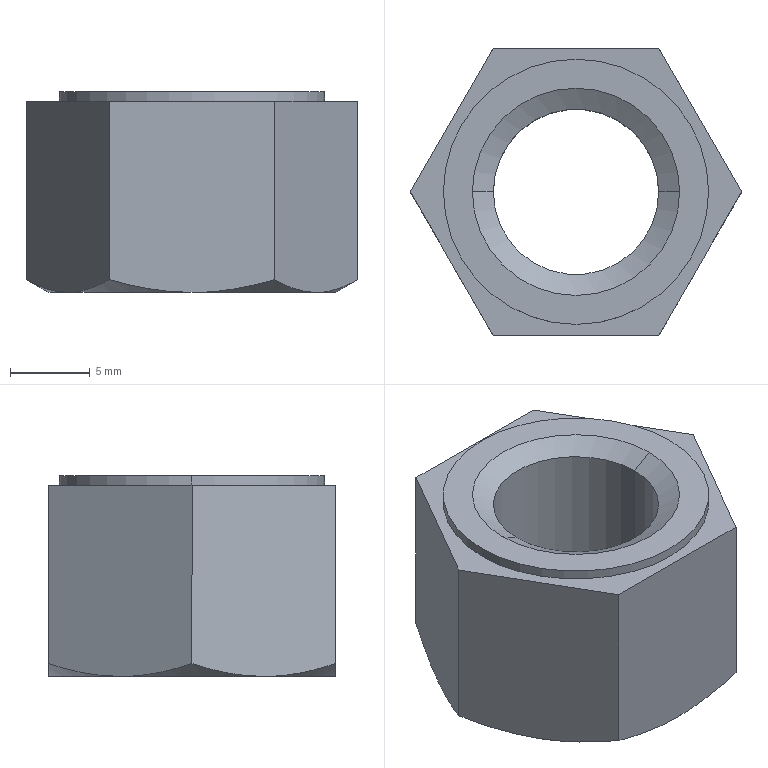Part | SolidWorks | features RevCut 4, Chamfer 2, Boss 1, Extrusion 1, LPattern 1 | 1 solid | 24 faces | box 20.785 x 18 x 12.6 mm | volume 2391 mm3 | cone 11 | plane 9 | cylinder 4 | commonest cylinder face diameters 10.376 x2 16.63 x2
STEP:
#1=CARTESIAN_POINT('',(-5.188,0.,-0.1575));
#2=VERTEX_POINT('',#1);
#3=CARTESIAN_POINT('',(5.188,0.,-0.1575));
#4=VERTEX_POINT('',#3);
#5=CARTESIAN_POINT('',(0.,0.,-0.1575));
#6=DIRECTION('',(0.,0.,1.));
#7=DIRECTION('',(1.,0.,0.));
#8=AXIS2_PLACEMENT_3D('',#5,#6,#7);
#9=CIRCLE('',#8,5.188);
#10=EDGE_CURVE('',#2,#4,#9,.T.);
#11=ORIENTED_EDGE('',*,*,#10,.F.);
#12=CARTESIAN_POINT('',(-6.5,0.,0.6));
#13=VERTEX_POINT('',#12);
#14=CARTESIAN_POINT('',(-5.188,0.,-0.1575));
#15=DIRECTION('',(-0.866,0.,0.5));
#16=VECTOR('',#15,1000.);
#17=LINE('',#14,#16);
#18=EDGE_CURVE('',#2,#13,#17,.T.);
#19=ORIENTED_EDGE('',*,*,#18,.T.);
#20=CARTESIAN_POINT('',(6.5,0.,0.6));
#21=VERTEX_POINT('',#20);
#22=CARTESIAN_POINT('',(0.,0.,0.6));
#23=DIRECTION('',(0.,0.,-1.));
#24=DIRECTION('',(1.,0.,0.));
#25=AXIS2_PLACEMENT_3D('',#22,#23,#24);
#26=CIRCLE('',#25,6.5);
#27=EDGE_CURVE('',#21,#13,#26,.T.);
#28=ORIENTED_EDGE('',*,*,#27,.F.);
#29=CARTESIAN_POINT('',(5.188,0.,-0.1575));
#30=DIRECTION('',(0.866,0.,0.5));
#31=VECTOR('',#30,1000.);
#32=LINE('',#29,#31);
#33=EDGE_CURVE('',#4,#21,#32,.T.);
#34=ORIENTED_EDGE('',*,*,#33,.F.);
#35=EDGE_LOOP('',(#11,#19,#28,#34));
#36=FACE_OUTER_BOUND('',#35,.T.);
#37=CARTESIAN_POINT('',(0.,0.,-0.1575));
#38=DIRECTION('',(0.,0.,1.));
#39=DIRECTION('',(1.,0.,0.));
#40=AXIS2_PLACEMENT_3D('',#37,#38,#39);
#41=CONICAL_SURFACE('',#40,5.188,1.047);
#42=ADVANCED_FACE('',(#36),#41,.F.);
#43=CARTESIAN_POINT('',(8.315,0.,0.6));
#44=VERTEX_POINT('',#43);
#45=CARTESIAN_POINT('',(-8.315,0.,0.6));
#46=VERTEX_POINT('',#45);
#47=CARTESIAN_POINT('',(0.,0.,0.6));
#48=DIRECTION('',(0.,0.,1.));
#49=DIRECTION('',(1.,0.,0.));
#50=AXIS2_PLACEMENT_3D('',#47,#48,#49);
#51=CIRCLE('',#50,8.315);
#52=EDGE_CURVE('',#44,#46,#51,.T.);
#53=ORIENTED_EDGE('',*,*,#52,.F.);
#54=CARTESIAN_POINT('',(8.315,0.,0.));
#55=VERTEX_POINT('',#54);
#56=CARTESIAN_POINT('',(8.315,0.,0.6));
#57=DIRECTION('',(0.,0.,-1.));
#58=VECTOR('',#57,1000.);
#59=LINE('',#56,#58);
#60=EDGE_CURVE('',#44,#55,#59,.T.);
#61=ORIENTED_EDGE('',*,*,#60,.T.);
#62=CARTESIAN_POINT('',(-8.315,0.,0.));
#63=VERTEX_POINT('',#62);
#64=CARTESIAN_POINT('',(0.,0.,0.));
#65=DIRECTION('',(0.,0.,1.));
#66=DIRECTION('',(1.,0.,0.));
#67=AXIS2_PLACEMENT_3D('',#64,#65,#66);
#68=CIRCLE('',#67,8.315);
#69=EDGE_CURVE('',#55,#63,#68,.T.);
#70=ORIENTED_EDGE('',*,*,#69,.T.);
#71=CARTESIAN_POINT('',(-8.315,0.,0.6));
#72=DIRECTION('',(0.,0.,-1.));
#73=VECTOR('',#72,1000.);
#74=LINE('',#71,#73);
#75=EDGE_CURVE('',#46,#63,#74,.T.);
#76=ORIENTED_EDGE('',*,*,#75,.F.);
#77=EDGE_LOOP('',(#53,#61,#70,#76));
#78=FACE_OUTER_BOUND('',#77,.T.);
#79=CARTESIAN_POINT('',(0.,0.,0.6));
#80=DIRECTION('',(0.,0.,-1.));
#81=DIRECTION('',(-1.,0.,0.));
#82=AXIS2_PLACEMENT_3D('',#79,#80,#81);
#83=CYLINDRICAL_SURFACE('',#82,8.315);
#84=ADVANCED_FACE('',(#78),#83,.T.);
#85=CARTESIAN_POINT('',(-5.188,0.,-11.243));
#86=VERTEX_POINT('',#85);
#87=CARTESIAN_POINT('',(5.188,0.,-11.243));
#88=VERTEX_POINT('',#87);
#89=CARTESIAN_POINT('',(0.,0.,-11.243));
#90=DIRECTION('',(0.,0.,1.));
#91=DIRECTION('',(1.,0.,0.));
#92=AXIS2_PLACEMENT_3D('',#89,#90,#91);
#93=CIRCLE('',#92,5.188);
#94=EDGE_CURVE('',#86,#88,#93,.T.);
#95=ORIENTED_EDGE('',*,*,#94,.T.);
#96=CARTESIAN_POINT('',(6.5,0.,-12.));
#97=VERTEX_POINT('',#96);
#98=CARTESIAN_POINT('',(5.188,0.,-11.243));
#99=DIRECTION('',(0.866,0.,-0.5));
#100=VECTOR('',#99,1000.);
#101=LINE('',#98,#100);
#102=EDGE_CURVE('',#88,#97,#101,.T.);
#103=ORIENTED_EDGE('',*,*,#102,.T.);
#104=CARTESIAN_POINT('',(-6.5,0.,-12.));
#105=VERTEX_POINT('',#104);
#106=CARTESIAN_POINT('',(0.,0.,-12.));
#107=DIRECTION('',(0.,0.,1.));
#108=DIRECTION('',(1.,0.,0.));
#109=AXIS2_PLACEMENT_3D('',#106,#107,#108);
#110=CIRCLE('',#109,6.5);
#111=EDGE_CURVE('',#105,#97,#110,.T.);
#112=ORIENTED_EDGE('',*,*,#111,.F.);
#113=CARTESIAN_POINT('',(-5.188,0.,-11.243));
#114=DIRECTION('',(-0.866,0.,-0.5));
#115=VECTOR('',#114,1000.);
#116=LINE('',#113,#115);
#117=EDGE_CURVE('',#86,#105,#116,.T.);
#118=ORIENTED_EDGE('',*,*,#117,.F.);
#119=EDGE_LOOP('',(#95,#103,#112,#118));
#120=FACE_OUTER_BOUND('',#119,.T.);
#121=CARTESIAN_POINT('',(0.,0.,-11.243));
#122=DIRECTION('',(0.,0.,-1.));
#123=DIRECTION('',(-1.,0.,0.));
#124=AXIS2_PLACEMENT_3D('',#121,#122,#123);
#125=CONICAL_SURFACE('',#124,5.188,1.047);
#126=ADVANCED_FACE('',(#120),#125,.F.);
#127=CARTESIAN_POINT('',(7.794,-4.5,-12.));
#128=VERTEX_POINT('',#127);
#129=CARTESIAN_POINT('',(9.,0.,-12.));
#130=VERTEX_POINT('',#129);
#131=CARTESIAN_POINT('',(0.,0.,-12.));
#132=DIRECTION('',(0.,0.,1.));
#133=DIRECTION('',(1.,0.,0.));
#134=AXIS2_PLACEMENT_3D('',#131,#132,#133);
#135=CIRCLE('',#134,9.);
#136=EDGE_CURVE('',#128,#130,#135,.T.);
#137=ORIENTED_EDGE('',*,*,#136,.T.);
#138=CARTESIAN_POINT('',(10.392,0.,-11.196));
#139=VERTEX_POINT('',#138);
#140=CARTESIAN_POINT('',(9.,0.,-12.));
#141=DIRECTION('',(0.866,0.,0.5));
#142=VECTOR('',#141,1000.);
#143=LINE('',#140,#142);
#144=EDGE_CURVE('',#130,#139,#143,.T.);
#145=ORIENTED_EDGE('',*,*,#144,.T.);
#146=CARTESIAN_POINT('',(7.794,-4.5,-12.));
#147=CARTESIAN_POINT('',(8.015,-4.118,-12.));
#148=CARTESIAN_POINT('',(8.236,-3.734,-11.981));
#149=CARTESIAN_POINT('',(8.674,-2.976,-11.907));
#150=CARTESIAN_POINT('',(8.892,-2.599,-11.853));
#151=CARTESIAN_POINT('',(9.541,-1.475,-11.643));
#152=CARTESIAN_POINT('',(9.968,-0.7343,-11.441));
#153=CARTESIAN_POINT('',(10.392,0.,-11.196));
#154=B_SPLINE_CURVE_WITH_KNOTS('',3,(#146,#147,#148,#149,#150,#151,#152,#153),.UNSPECIFIED.,.F.,.F.,(4,2,2,4),(0.005258,0.006567,0.007877,0.0105),.UNSPECIFIED.);
#155=EDGE_CURVE('',#128,#139,#154,.T.);
#156=ORIENTED_EDGE('',*,*,#155,.F.);
#157=EDGE_LOOP('',(#137,#145,#156));
#158=FACE_OUTER_BOUND('',#157,.T.);
#159=CARTESIAN_POINT('',(0.,0.,-12.));
#160=DIRECTION('',(0.,0.,1.));
#161=DIRECTION('',(1.,0.,0.));
#162=AXIS2_PLACEMENT_3D('',#159,#160,#161);
#163=CONICAL_SURFACE('',#162,9.,1.047);
#164=ADVANCED_FACE('',(#158),#163,.T.);
#165=ORIENTED_EDGE('',*,*,#94,.F.);
#166=CARTESIAN_POINT('',(-5.188,0.,-12.));
#167=DIRECTION('',(0.,0.,1.));
#168=VECTOR('',#167,1000.);
#169=LINE('',#166,#168);
#170=EDGE_CURVE('',#86,#2,#169,.T.);
#171=ORIENTED_EDGE('',*,*,#170,.T.);
#172=ORIENTED_EDGE('',*,*,#10,.T.);
#173=CARTESIAN_POINT('',(5.188,0.,-12.));
#174=DIRECTION('',(0.,0.,1.));
#175=VECTOR('',#174,1000.);
#176=LINE('',#173,#175);
#177=EDGE_CURVE('',#88,#4,#176,.T.);
#178=ORIENTED_EDGE('',*,*,#177,.F.);
#179=EDGE_LOOP('',(#165,#171,#172,#178));
#180=FACE_OUTER_BOUND('',#179,.T.);
#181=CARTESIAN_POINT('',(0.,0.,-12.));
#182=DIRECTION('',(0.,0.,1.));
#183=DIRECTION('',(1.,0.,0.));
#184=AXIS2_PLACEMENT_3D('',#181,#182,#183);
#185=CYLINDRICAL_SURFACE('',#184,5.188);
#186=ADVANCED_FACE('',(#180),#185,.F.);
#187=CARTESIAN_POINT('',(-5.196,-9.,0.));
#188=VERTEX_POINT('',#187);
#189=CARTESIAN_POINT('',(5.196,-9.,0.));
#190=VERTEX_POINT('',#189);
#191=CARTESIAN_POINT('',(-5.196,-9.,0.));
#192=DIRECTION('',(1.,0.,0.));
#193=VECTOR('',#192,1000.);
#194=LINE('',#191,#193);
#195=EDGE_CURVE('',#188,#190,#194,.T.);
#196=ORIENTED_EDGE('',*,*,#195,.T.);
#197=CARTESIAN_POINT('',(10.392,0.,0.));
#198=VERTEX_POINT('',#197);
#199=CARTESIAN_POINT('',(5.196,-9.,0.));
#200=DIRECTION('',(0.5,0.866,0.));
#201=VECTOR('',#200,1000.);
#202=LINE('',#199,#201);
#203=EDGE_CURVE('',#190,#198,#202,.T.);
#204=ORIENTED_EDGE('',*,*,#203,.T.);
#205=CARTESIAN_POINT('',(5.196,9.,0.));
#206=VERTEX_POINT('',#205);
#207=CARTESIAN_POINT('',(10.392,0.,0.));
#208=DIRECTION('',(-0.5,0.866,0.));
#209=VECTOR('',#208,1000.);
#210=LINE('',#207,#209);
#211=EDGE_CURVE('',#198,#206,#210,.T.);
#212=ORIENTED_EDGE('',*,*,#211,.T.);
#213=CARTESIAN_POINT('',(-5.196,9.,0.));
#214=VERTEX_POINT('',#213);
#215=CARTESIAN_POINT('',(5.196,9.,0.));
#216=DIRECTION('',(-1.,0.,0.));
#217=VECTOR('',#216,1000.);
#218=LINE('',#215,#217);
#219=EDGE_CURVE('',#206,#214,#218,.T.);
#220=ORIENTED_EDGE('',*,*,#219,.T.);
#221=CARTESIAN_POINT('',(-10.392,0.,0.));
#222=VERTEX_POINT('',#221);
#223=CARTESIAN_POINT('',(-5.196,9.,0.));
#224=DIRECTION('',(-0.5,-0.866,0.));
#225=VECTOR('',#224,1000.);
#226=LINE('',#223,#225);
#227=EDGE_CURVE('',#214,#222,#226,.T.);
#228=ORIENTED_EDGE('',*,*,#227,.T.);
#229=CARTESIAN_POINT('',(-10.392,0.,0.));
#230=DIRECTION('',(0.5,-0.866,0.));
#231=VECTOR('',#230,1000.);
#232=LINE('',#229,#231);
#233=EDGE_CURVE('',#222,#188,#232,.T.);
#234=ORIENTED_EDGE('',*,*,#233,.T.);
#235=EDGE_LOOP('',(#196,#204,#212,#220,#228,#234));
#236=FACE_OUTER_BOUND('',#235,.T.);
#237=CARTESIAN_POINT('',(0.,0.,0.));
#238=DIRECTION('',(0.,0.,1.));
#239=DIRECTION('',(1.,0.,0.));
#240=AXIS2_PLACEMENT_3D('',#237,#238,#239);
#241=CIRCLE('',#240,8.315);
#242=EDGE_CURVE('',#63,#55,#241,.T.);
#243=ORIENTED_EDGE('',*,*,#242,.F.);
#244=ORIENTED_EDGE('',*,*,#69,.F.);
#245=EDGE_LOOP('',(#243,#244));
#246=FACE_BOUND('',#245,.T.);
#247=CARTESIAN_POINT('',(5.196,-9.,0.));
#248=DIRECTION('',(0.,0.,1.));
#249=DIRECTION('',(1.,0.,0.));
#250=AXIS2_PLACEMENT_3D('',#247,#248,#249);
#251=PLANE('',#250);
#252=ADVANCED_FACE('',(#236,#246),#251,.T.);
#253=CARTESIAN_POINT('',(-5.196,-9.,-11.196));
#254=VERTEX_POINT('',#253);
#255=CARTESIAN_POINT('',(-5.196,-9.,-12.));
#256=DIRECTION('',(0.,0.,1.));
#257=VECTOR('',#256,1000.);
#258=LINE('',#255,#257);
#259=EDGE_CURVE('',#254,#188,#258,.T.);
#260=ORIENTED_EDGE('',*,*,#259,.F.);
#261=CARTESIAN_POINT('',(0.,-9.,-12.));
#262=VERTEX_POINT('',#261);
#263=CARTESIAN_POINT('',(-5.196,-9.,-11.196));
#264=CARTESIAN_POINT('',(-4.351,-9.,-11.44));
#265=CARTESIAN_POINT('',(-3.485,-9.,-11.645));
#266=CARTESIAN_POINT('',(-1.75,-9.,-11.925));
#267=CARTESIAN_POINT('',(-0.8781,-9.,-12.));
#268=CARTESIAN_POINT('',(0.,-9.,-12.));
#269=B_SPLINE_CURVE_WITH_KNOTS('',3,(#263,#264,#265,#266,#267,#268),.UNSPECIFIED.,.F.,.F.,(4,2,4),(0.009271,0.0119,0.01453),.UNSPECIFIED.);
#270=EDGE_CURVE('',#254,#262,#269,.T.);
#271=ORIENTED_EDGE('',*,*,#270,.T.);
#272=CARTESIAN_POINT('',(5.196,-9.,-11.196));
#273=VERTEX_POINT('',#272);
#274=CARTESIAN_POINT('',(0.,-9.,-12.));
#275=CARTESIAN_POINT('',(0.8786,-9.,-12.));
#276=CARTESIAN_POINT('',(1.769,-9.,-11.922));
#277=CARTESIAN_POINT('',(3.505,-9.,-11.641));
#278=CARTESIAN_POINT('',(4.356,-9.,-11.439));
#279=CARTESIAN_POINT('',(5.196,-9.,-11.196));
#280=B_SPLINE_CURVE_WITH_KNOTS('',3,(#274,#275,#276,#277,#278,#279),.UNSPECIFIED.,.F.,.F.,(4,2,4),(0.01453,0.01716,0.01979),.UNSPECIFIED.);
#281=EDGE_CURVE('',#262,#273,#280,.T.);
#282=ORIENTED_EDGE('',*,*,#281,.T.);
#283=CARTESIAN_POINT('',(5.196,-9.,-12.));
#284=DIRECTION('',(0.,0.,1.));
#285=VECTOR('',#284,1000.);
#286=LINE('',#283,#285);
#287=EDGE_CURVE('',#273,#190,#286,.T.);
#288=ORIENTED_EDGE('',*,*,#287,.T.);
#289=ORIENTED_EDGE('',*,*,#195,.F.);
#290=EDGE_LOOP('',(#260,#271,#282,#288,#289));
#291=FACE_OUTER_BOUND('',#290,.T.);
#292=CARTESIAN_POINT('',(-5.196,-9.,-12.));
#293=DIRECTION('',(0.,-1.,0.));
#294=DIRECTION('',(1.,0.,0.));
#295=AXIS2_PLACEMENT_3D('',#292,#293,#294);
#296=PLANE('',#295);
#297=ADVANCED_FACE('',(#291),#296,.T.);
#298=CARTESIAN_POINT('',(-10.392,0.,-11.196));
#299=VERTEX_POINT('',#298);
#300=CARTESIAN_POINT('',(-10.392,0.,-12.));
#301=DIRECTION('',(0.,0.,1.));
#302=VECTOR('',#301,1000.);
#303=LINE('',#300,#302);
#304=EDGE_CURVE('',#299,#222,#303,.T.);
#305=ORIENTED_EDGE('',*,*,#304,.F.);
#306=CARTESIAN_POINT('',(-7.794,-4.5,-12.));
#307=VERTEX_POINT('',#306);
#308=CARTESIAN_POINT('',(-10.392,0.,-11.196));
#309=CARTESIAN_POINT('',(-9.967,-0.7361,-11.442));
#310=CARTESIAN_POINT('',(-9.539,-1.478,-11.644));
#311=CARTESIAN_POINT('',(-8.674,-2.976,-11.923));
#312=CARTESIAN_POINT('',(-8.237,-3.733,-12.));
#313=CARTESIAN_POINT('',(-7.794,-4.5,-12.));
#314=B_SPLINE_CURVE_WITH_KNOTS('',3,(#308,#309,#310,#311,#312,#313),.UNSPECIFIED.,.F.,.F.,(4,2,4),(0.000000238,0.002629,0.005258),.UNSPECIFIED.);
#315=EDGE_CURVE('',#299,#307,#314,.T.);
#316=ORIENTED_EDGE('',*,*,#315,.T.);
#317=CARTESIAN_POINT('',(-7.794,-4.5,-12.));
#318=CARTESIAN_POINT('',(-7.574,-4.882,-12.));
#319=CARTESIAN_POINT('',(-7.352,-5.266,-11.981));
#320=CARTESIAN_POINT('',(-6.914,-6.024,-11.907));
#321=CARTESIAN_POINT('',(-6.697,-6.401,-11.853));
#322=CARTESIAN_POINT('',(-6.048,-7.525,-11.643));
#323=CARTESIAN_POINT('',(-5.62,-8.266,-11.441));
#324=CARTESIAN_POINT('',(-5.196,-9.,-11.196));
#325=B_SPLINE_CURVE_WITH_KNOTS('',3,(#317,#318,#319,#320,#321,#322,#323,#324),.UNSPECIFIED.,.F.,.F.,(4,2,2,4),(0.005258,0.006567,0.007877,0.0105),.UNSPECIFIED.);
#326=EDGE_CURVE('',#307,#254,#325,.T.);
#327=ORIENTED_EDGE('',*,*,#326,.T.);
#328=ORIENTED_EDGE('',*,*,#259,.T.);
#329=ORIENTED_EDGE('',*,*,#233,.F.);
#330=EDGE_LOOP('',(#305,#316,#327,#328,#329));
#331=FACE_OUTER_BOUND('',#330,.T.);
#332=CARTESIAN_POINT('',(-10.392,0.,-12.));
#333=DIRECTION('',(-0.866,-0.5,0.));
#334=DIRECTION('',(0.5,-0.866,0.));
#335=AXIS2_PLACEMENT_3D('',#332,#333,#334);
#336=PLANE('',#335);
#337=ADVANCED_FACE('',(#331),#336,.T.);
#338=CARTESIAN_POINT('',(-5.196,9.,-11.196));
#339=VERTEX_POINT('',#338);
#340=CARTESIAN_POINT('',(-5.196,9.,-12.));
#341=DIRECTION('',(0.,0.,1.));
#342=VECTOR('',#341,1000.);
#343=LINE('',#340,#342);
#344=EDGE_CURVE('',#339,#214,#343,.T.);
#345=ORIENTED_EDGE('',*,*,#344,.F.);
#346=CARTESIAN_POINT('',(-7.794,4.5,-12.));
#347=VERTEX_POINT('',#346);
#348=CARTESIAN_POINT('',(-5.196,9.,-11.196));
#349=CARTESIAN_POINT('',(-5.621,8.264,-11.442));
#350=CARTESIAN_POINT('',(-6.049,7.522,-11.644));
#351=CARTESIAN_POINT('',(-6.914,6.024,-11.923));
#352=CARTESIAN_POINT('',(-7.352,5.267,-12.));
#353=CARTESIAN_POINT('',(-7.794,4.5,-12.));
#354=B_SPLINE_CURVE_WITH_KNOTS('',3,(#348,#349,#350,#351,#352,#353),.UNSPECIFIED.,.F.,.F.,(4,2,4),(0.000000238,0.002629,0.005258),.UNSPECIFIED.);
#355=EDGE_CURVE('',#339,#347,#354,.T.);
#356=ORIENTED_EDGE('',*,*,#355,.T.);
#357=CARTESIAN_POINT('',(-7.794,4.5,-12.));
#358=CARTESIAN_POINT('',(-8.015,4.118,-12.));
#359=CARTESIAN_POINT('',(-8.236,3.734,-11.981));
#360=CARTESIAN_POINT('',(-8.674,2.976,-11.907));
#361=CARTESIAN_POINT('',(-8.892,2.599,-11.853));
#362=CARTESIAN_POINT('',(-9.541,1.475,-11.643));
#363=CARTESIAN_POINT('',(-9.968,0.7343,-11.441));
#364=CARTESIAN_POINT('',(-10.392,0.,-11.196));
#365=B_SPLINE_CURVE_WITH_KNOTS('',3,(#357,#358,#359,#360,#361,#362,#363,#364),.UNSPECIFIED.,.F.,.F.,(4,2,2,4),(0.005258,0.006567,0.007877,0.0105),.UNSPECIFIED.);
#366=EDGE_CURVE('',#347,#299,#365,.T.);
#367=ORIENTED_EDGE('',*,*,#366,.T.);
#368=ORIENTED_EDGE('',*,*,#304,.T.);
#369=ORIENTED_EDGE('',*,*,#227,.F.);
#370=EDGE_LOOP('',(#345,#356,#367,#368,#369));
#371=FACE_OUTER_BOUND('',#370,.T.);
#372=CARTESIAN_POINT('',(-5.196,9.,-12.));
#373=DIRECTION('',(-0.866,0.5,0.));
#374=DIRECTION('',(-0.5,-0.866,0.));
#375=AXIS2_PLACEMENT_3D('',#372,#373,#374);
#376=PLANE('',#375);
#377=ADVANCED_FACE('',(#371),#376,.T.);
#378=CARTESIAN_POINT('',(5.196,9.,-11.196));
#379=VERTEX_POINT('',#378);
#380=CARTESIAN_POINT('',(5.196,9.,-12.));
#381=DIRECTION('',(0.,0.,1.));
#382=VECTOR('',#381,1000.);
#383=LINE('',#380,#382);
#384=EDGE_CURVE('',#379,#206,#383,.T.);
#385=ORIENTED_EDGE('',*,*,#384,.F.);
#386=CARTESIAN_POINT('',(0.,9.,-12.));
#387=VERTEX_POINT('',#386);
#388=CARTESIAN_POINT('',(5.196,9.,-11.196));
#389=CARTESIAN_POINT('',(4.356,9.,-11.439));
#390=CARTESIAN_POINT('',(3.505,9.,-11.641));
#391=CARTESIAN_POINT('',(1.769,9.,-11.922));
#392=CARTESIAN_POINT('',(0.8786,9.,-12.));
#393=CARTESIAN_POINT('',(0.,9.,-12.));
#394=B_SPLINE_CURVE_WITH_KNOTS('',3,(#388,#389,#390,#391,#392,#393),.UNSPECIFIED.,.F.,.F.,(4,2,4),(0.003809,0.006432,0.009055),.UNSPECIFIED.);
#395=EDGE_CURVE('',#379,#387,#394,.T.);
#396=ORIENTED_EDGE('',*,*,#395,.T.);
#397=CARTESIAN_POINT('',(0.,9.,-12.));
#398=CARTESIAN_POINT('',(-0.8781,9.,-12.));
#399=CARTESIAN_POINT('',(-1.75,9.,-11.925));
#400=CARTESIAN_POINT('',(-3.485,9.,-11.645));
#401=CARTESIAN_POINT('',(-4.351,9.,-11.44));
#402=CARTESIAN_POINT('',(-5.196,9.,-11.196));
#403=B_SPLINE_CURVE_WITH_KNOTS('',3,(#397,#398,#399,#400,#401,#402),.UNSPECIFIED.,.F.,.F.,(4,2,4),(0.009055,0.01168,0.0143),.UNSPECIFIED.);
#404=EDGE_CURVE('',#387,#339,#403,.T.);
#405=ORIENTED_EDGE('',*,*,#404,.T.);
#406=ORIENTED_EDGE('',*,*,#344,.T.);
#407=ORIENTED_EDGE('',*,*,#219,.F.);
#408=EDGE_LOOP('',(#385,#396,#405,#406,#407));
#409=FACE_OUTER_BOUND('',#408,.T.);
#410=CARTESIAN_POINT('',(5.196,9.,-12.));
#411=DIRECTION('',(0.,1.,0.));
#412=DIRECTION('',(0.,0.,1.));
#413=AXIS2_PLACEMENT_3D('',#410,#411,#412);
#414=PLANE('',#413);
#415=ADVANCED_FACE('',(#409),#414,.T.);
#416=CARTESIAN_POINT('',(10.392,0.,-12.));
#417=DIRECTION('',(0.,0.,1.));
#418=VECTOR('',#417,1000.);
#419=LINE('',#416,#418);
#420=EDGE_CURVE('',#139,#198,#419,.T.);
#421=ORIENTED_EDGE('',*,*,#420,.F.);
#422=CARTESIAN_POINT('',(7.794,4.5,-12.));
#423=VERTEX_POINT('',#422);
#424=CARTESIAN_POINT('',(10.392,0.,-11.196));
#425=CARTESIAN_POINT('',(9.967,0.7361,-11.442));
#426=CARTESIAN_POINT('',(9.539,1.478,-11.644));
#427=CARTESIAN_POINT('',(8.674,2.976,-11.923));
#428=CARTESIAN_POINT('',(8.237,3.733,-12.));
#429=CARTESIAN_POINT('',(7.794,4.5,-12.));
#430=B_SPLINE_CURVE_WITH_KNOTS('',3,(#424,#425,#426,#427,#428,#429),.UNSPECIFIED.,.F.,.F.,(4,2,4),(0.000000238,0.002629,0.005258),.UNSPECIFIED.);
#431=EDGE_CURVE('',#139,#423,#430,.T.);
#432=ORIENTED_EDGE('',*,*,#431,.T.);
#433=CARTESIAN_POINT('',(7.794,4.5,-12.));
#434=CARTESIAN_POINT('',(7.574,4.882,-12.));
#435=CARTESIAN_POINT('',(7.352,5.266,-11.981));
#436=CARTESIAN_POINT('',(6.914,6.024,-11.907));
#437=CARTESIAN_POINT('',(6.697,6.401,-11.853));
#438=CARTESIAN_POINT('',(6.048,7.525,-11.643));
#439=CARTESIAN_POINT('',(5.62,8.266,-11.441));
#440=CARTESIAN_POINT('',(5.196,9.,-11.196));
#441=B_SPLINE_CURVE_WITH_KNOTS('',3,(#433,#434,#435,#436,#437,#438,#439,#440),.UNSPECIFIED.,.F.,.F.,(4,2,2,4),(0.005258,0.006567,0.007877,0.0105),.UNSPECIFIED.);
#442=EDGE_CURVE('',#423,#379,#441,.T.);
#443=ORIENTED_EDGE('',*,*,#442,.T.);
#444=ORIENTED_EDGE('',*,*,#384,.T.);
#445=ORIENTED_EDGE('',*,*,#211,.F.);
#446=EDGE_LOOP('',(#421,#432,#443,#444,#445));
#447=FACE_OUTER_BOUND('',#446,.T.);
#448=CARTESIAN_POINT('',(10.392,0.,-12.));
#449=DIRECTION('',(0.866,0.5,0.));
#450=DIRECTION('',(-0.5,0.866,0.));
#451=AXIS2_PLACEMENT_3D('',#448,#449,#450);
#452=PLANE('',#451);
#453=ADVANCED_FACE('',(#447),#452,.T.);
#454=ORIENTED_EDGE('',*,*,#287,.F.);
#455=CARTESIAN_POINT('',(5.196,-9.,-11.196));
#456=CARTESIAN_POINT('',(5.621,-8.264,-11.442));
#457=CARTESIAN_POINT('',(6.049,-7.522,-11.644));
#458=CARTESIAN_POINT('',(6.914,-6.024,-11.923));
#459=CARTESIAN_POINT('',(7.352,-5.267,-12.));
#460=CARTESIAN_POINT('',(7.794,-4.5,-12.));
#461=B_SPLINE_CURVE_WITH_KNOTS('',3,(#455,#456,#457,#458,#459,#460),.UNSPECIFIED.,.F.,.F.,(4,2,4),(0.000000238,0.002629,0.005258),.UNSPECIFIED.);
#462=EDGE_CURVE('',#273,#128,#461,.T.);
#463=ORIENTED_EDGE('',*,*,#462,.T.);
#464=ORIENTED_EDGE('',*,*,#155,.T.);
#465=ORIENTED_EDGE('',*,*,#420,.T.);
#466=ORIENTED_EDGE('',*,*,#203,.F.);
#467=EDGE_LOOP('',(#454,#463,#464,#465,#466));
#468=FACE_OUTER_BOUND('',#467,.T.);
#469=CARTESIAN_POINT('',(5.196,-9.,-12.));
#470=DIRECTION('',(0.866,-0.5,0.));
#471=DIRECTION('',(0.5,0.866,0.));
#472=AXIS2_PLACEMENT_3D('',#469,#470,#471);
#473=PLANE('',#472);
#474=ADVANCED_FACE('',(#468),#473,.T.);
#475=ORIENTED_EDGE('',*,*,#111,.T.);
#476=CARTESIAN_POINT('',(0.,0.,-12.));
#477=DIRECTION('',(0.,0.,1.));
#478=DIRECTION('',(1.,0.,0.));
#479=AXIS2_PLACEMENT_3D('',#476,#477,#478);
#480=CIRCLE('',#479,6.5);
#481=EDGE_CURVE('',#97,#105,#480,.T.);
#482=ORIENTED_EDGE('',*,*,#481,.T.);
#483=EDGE_LOOP('',(#475,#482));
#484=FACE_BOUND('',#483,.T.);
#485=CARTESIAN_POINT('',(0.,0.,-12.));
#486=DIRECTION('',(0.,0.,1.));
#487=DIRECTION('',(1.,0.,0.));
#488=AXIS2_PLACEMENT_3D('',#485,#486,#487);
#489=CIRCLE('',#488,9.);
#490=EDGE_CURVE('',#423,#387,#489,.T.);
#491=ORIENTED_EDGE('',*,*,#490,.F.);
#492=CARTESIAN_POINT('',(0.,0.,-12.));
#493=DIRECTION('',(0.,0.,1.));
#494=DIRECTION('',(1.,0.,0.));
#495=AXIS2_PLACEMENT_3D('',#492,#493,#494);
#496=CIRCLE('',#495,9.);
#497=EDGE_CURVE('',#130,#423,#496,.T.);
#498=ORIENTED_EDGE('',*,*,#497,.F.);
#499=ORIENTED_EDGE('',*,*,#136,.F.);
#500=CARTESIAN_POINT('',(0.,0.,-12.));
#501=DIRECTION('',(0.,0.,1.));
#502=DIRECTION('',(1.,0.,0.));
#503=AXIS2_PLACEMENT_3D('',#500,#501,#502);
#504=CIRCLE('',#503,9.);
#505=EDGE_CURVE('',#262,#128,#504,.T.);
#506=ORIENTED_EDGE('',*,*,#505,.F.);
#507=CARTESIAN_POINT('',(0.,0.,-12.));
#508=DIRECTION('',(0.,0.,1.));
#509=DIRECTION('',(1.,0.,0.));
#510=AXIS2_PLACEMENT_3D('',#507,#508,#509);
#511=CIRCLE('',#510,9.);
#512=EDGE_CURVE('',#307,#262,#511,.T.);
#513=ORIENTED_EDGE('',*,*,#512,.F.);
#514=CARTESIAN_POINT('',(0.,0.,-12.));
#515=DIRECTION('',(0.,0.,1.));
#516=DIRECTION('',(1.,0.,0.));
#517=AXIS2_PLACEMENT_3D('',#514,#515,#516);
#518=CIRCLE('',#517,9.);
#519=EDGE_CURVE('',#347,#307,#518,.T.);
#520=ORIENTED_EDGE('',*,*,#519,.F.);
#521=CARTESIAN_POINT('',(0.,0.,-12.));
#522=DIRECTION('',(0.,0.,-1.));
#523=DIRECTION('',(-1.,0.,0.));
#524=AXIS2_PLACEMENT_3D('',#521,#522,#523);
#525=CIRCLE('',#524,9.);
#526=EDGE_CURVE('',#347,#387,#525,.T.);
#527=ORIENTED_EDGE('',*,*,#526,.T.);
#528=EDGE_LOOP('',(#491,#498,#499,#506,#513,#520,#527));
#529=FACE_OUTER_BOUND('',#528,.T.);
#530=CARTESIAN_POINT('',(5.196,-9.,-12.));
#531=DIRECTION('',(0.,0.,1.));
#532=DIRECTION('',(1.,0.,0.));
#533=AXIS2_PLACEMENT_3D('',#530,#531,#532);
#534=PLANE('',#533);
#535=ADVANCED_FACE('',(#484,#529),#534,.F.);
#536=ORIENTED_EDGE('',*,*,#170,.F.);
#537=CARTESIAN_POINT('',(0.,0.,-11.243));
#538=DIRECTION('',(0.,0.,1.));
#539=DIRECTION('',(1.,0.,0.));
#540=AXIS2_PLACEMENT_3D('',#537,#538,#539);
#541=CIRCLE('',#540,5.188);
#542=EDGE_CURVE('',#88,#86,#541,.T.);
#543=ORIENTED_EDGE('',*,*,#542,.F.);
#544=ORIENTED_EDGE('',*,*,#177,.T.);
#545=CARTESIAN_POINT('',(0.,0.,-0.1575));
#546=DIRECTION('',(0.,0.,1.));
#547=DIRECTION('',(1.,0.,0.));
#548=AXIS2_PLACEMENT_3D('',#545,#546,#547);
#549=CIRCLE('',#548,5.188);
#550=EDGE_CURVE('',#4,#2,#549,.T.);
#551=ORIENTED_EDGE('',*,*,#550,.T.);
#552=EDGE_LOOP('',(#536,#543,#544,#551));
#553=FACE_OUTER_BOUND('',#552,.T.);
#554=CARTESIAN_POINT('',(0.,0.,-12.));
#555=DIRECTION('',(0.,0.,1.));
#556=DIRECTION('',(1.,0.,0.));
#557=AXIS2_PLACEMENT_3D('',#554,#555,#556);
#558=CYLINDRICAL_SURFACE('',#557,5.188);
#559=ADVANCED_FACE('',(#553),#558,.F.);
#560=ORIENTED_EDGE('',*,*,#144,.F.);
#561=ORIENTED_EDGE('',*,*,#497,.T.);
#562=ORIENTED_EDGE('',*,*,#431,.F.);
#563=EDGE_LOOP('',(#560,#561,#562));
#564=FACE_OUTER_BOUND('',#563,.T.);
#565=CARTESIAN_POINT('',(0.,0.,-12.));
#566=DIRECTION('',(0.,0.,1.));
#567=DIRECTION('',(1.,0.,0.));
#568=AXIS2_PLACEMENT_3D('',#565,#566,#567);
#569=CONICAL_SURFACE('',#568,9.,1.047);
#570=ADVANCED_FACE('',(#564),#569,.T.);
#571=ORIENTED_EDGE('',*,*,#505,.T.);
#572=ORIENTED_EDGE('',*,*,#462,.F.);
#573=ORIENTED_EDGE('',*,*,#281,.F.);
#574=EDGE_LOOP('',(#571,#572,#573));
#575=FACE_OUTER_BOUND('',#574,.T.);
#576=CARTESIAN_POINT('',(0.,0.,-12.));
#577=DIRECTION('',(0.,0.,1.));
#578=DIRECTION('',(1.,0.,0.));
#579=AXIS2_PLACEMENT_3D('',#576,#577,#578);
#580=CONICAL_SURFACE('',#579,9.,1.047);
#581=ADVANCED_FACE('',(#575),#580,.T.);
#582=ORIENTED_EDGE('',*,*,#512,.T.);
#583=ORIENTED_EDGE('',*,*,#270,.F.);
#584=ORIENTED_EDGE('',*,*,#326,.F.);
#585=EDGE_LOOP('',(#582,#583,#584));
#586=FACE_OUTER_BOUND('',#585,.T.);
#587=CARTESIAN_POINT('',(0.,0.,-12.));
#588=DIRECTION('',(0.,0.,1.));
#589=DIRECTION('',(1.,0.,0.));
#590=AXIS2_PLACEMENT_3D('',#587,#588,#589);
#591=CONICAL_SURFACE('',#590,9.,1.047);
#592=ADVANCED_FACE('',(#586),#591,.T.);
#593=ORIENTED_EDGE('',*,*,#519,.T.);
#594=ORIENTED_EDGE('',*,*,#315,.F.);
#595=ORIENTED_EDGE('',*,*,#366,.F.);
#596=EDGE_LOOP('',(#593,#594,#595));
#597=FACE_OUTER_BOUND('',#596,.T.);
#598=CARTESIAN_POINT('',(0.,0.,-12.));
#599=DIRECTION('',(0.,0.,1.));
#600=DIRECTION('',(1.,0.,0.));
#601=AXIS2_PLACEMENT_3D('',#598,#599,#600);
#602=CONICAL_SURFACE('',#601,9.,1.047);
#603=ADVANCED_FACE('',(#597),#602,.T.);
#604=ORIENTED_EDGE('',*,*,#404,.F.);
#605=ORIENTED_EDGE('',*,*,#526,.F.);
#606=ORIENTED_EDGE('',*,*,#355,.F.);
#607=EDGE_LOOP('',(#604,#605,#606));
#608=FACE_OUTER_BOUND('',#607,.T.);
#609=CARTESIAN_POINT('',(0.,0.,-12.));
#610=DIRECTION('',(0.,0.,1.));
#611=DIRECTION('',(1.,0.,0.));
#612=AXIS2_PLACEMENT_3D('',#609,#610,#611);
#613=CONICAL_SURFACE('',#612,9.,1.047);
#614=ADVANCED_FACE('',(#608),#613,.T.);
#615=ORIENTED_EDGE('',*,*,#442,.F.);
#616=ORIENTED_EDGE('',*,*,#490,.T.);
#617=ORIENTED_EDGE('',*,*,#395,.F.);
#618=EDGE_LOOP('',(#615,#616,#617));
#619=FACE_OUTER_BOUND('',#618,.T.);
#620=CARTESIAN_POINT('',(0.,0.,-12.));
#621=DIRECTION('',(0.,0.,1.));
#622=DIRECTION('',(1.,0.,0.));
#623=AXIS2_PLACEMENT_3D('',#620,#621,#622);
#624=CONICAL_SURFACE('',#623,9.,1.047);
#625=ADVANCED_FACE('',(#619),#624,.T.);
#626=ORIENTED_EDGE('',*,*,#102,.F.);
#627=ORIENTED_EDGE('',*,*,#542,.T.);
#628=ORIENTED_EDGE('',*,*,#117,.T.);
#629=ORIENTED_EDGE('',*,*,#481,.F.);
#630=EDGE_LOOP('',(#626,#627,#628,#629));
#631=FACE_OUTER_BOUND('',#630,.T.);
#632=CARTESIAN_POINT('',(0.,0.,-11.243));
#633=DIRECTION('',(0.,0.,-1.));
#634=DIRECTION('',(-1.,0.,0.));
#635=AXIS2_PLACEMENT_3D('',#632,#633,#634);
#636=CONICAL_SURFACE('',#635,5.188,1.047);
#637=ADVANCED_FACE('',(#631),#636,.F.);
#638=ORIENTED_EDGE('',*,*,#27,.T.);
#639=CARTESIAN_POINT('',(0.,0.,0.6));
#640=DIRECTION('',(0.,0.,-1.));
#641=DIRECTION('',(1.,0.,0.));
#642=AXIS2_PLACEMENT_3D('',#639,#640,#641);
#643=CIRCLE('',#642,6.5);
#644=EDGE_CURVE('',#13,#21,#643,.T.);
#645=ORIENTED_EDGE('',*,*,#644,.T.);
#646=EDGE_LOOP('',(#638,#645));
#647=FACE_BOUND('',#646,.T.);
#648=CARTESIAN_POINT('',(0.,0.,0.6));
#649=DIRECTION('',(0.,0.,1.));
#650=DIRECTION('',(1.,0.,0.));
#651=AXIS2_PLACEMENT_3D('',#648,#649,#650);
#652=CIRCLE('',#651,8.315);
#653=EDGE_CURVE('',#46,#44,#652,.T.);
#654=ORIENTED_EDGE('',*,*,#653,.T.);
#655=ORIENTED_EDGE('',*,*,#52,.T.);
#656=EDGE_LOOP('',(#654,#655));
#657=FACE_OUTER_BOUND('',#656,.T.);
#658=CARTESIAN_POINT('',(0.,0.,0.6));
#659=DIRECTION('',(0.,0.,1.));
#660=DIRECTION('',(1.,0.,0.));
#661=AXIS2_PLACEMENT_3D('',#658,#659,#660);
#662=PLANE('',#661);
#663=ADVANCED_FACE('',(#647,#657),#662,.T.);
#664=ORIENTED_EDGE('',*,*,#60,.F.);
#665=ORIENTED_EDGE('',*,*,#653,.F.);
#666=ORIENTED_EDGE('',*,*,#75,.T.);
#667=ORIENTED_EDGE('',*,*,#242,.T.);
#668=EDGE_LOOP('',(#664,#665,#666,#667));
#669=FACE_OUTER_BOUND('',#668,.T.);
#670=CARTESIAN_POINT('',(0.,0.,0.6));
#671=DIRECTION('',(0.,0.,-1.));
#672=DIRECTION('',(-1.,0.,0.));
#673=AXIS2_PLACEMENT_3D('',#670,#671,#672);
#674=CYLINDRICAL_SURFACE('',#673,8.315);
#675=ADVANCED_FACE('',(#669),#674,.T.);
#676=ORIENTED_EDGE('',*,*,#18,.F.);
#677=ORIENTED_EDGE('',*,*,#550,.F.);
#678=ORIENTED_EDGE('',*,*,#33,.T.);
#679=ORIENTED_EDGE('',*,*,#644,.F.);
#680=EDGE_LOOP('',(#676,#677,#678,#679));
#681=FACE_OUTER_BOUND('',#680,.T.);
#682=CARTESIAN_POINT('',(0.,0.,-0.1575));
#683=DIRECTION('',(0.,0.,1.));
#684=DIRECTION('',(1.,0.,0.));
#685=AXIS2_PLACEMENT_3D('',#682,#683,#684);
#686=CONICAL_SURFACE('',#685,5.188,1.047);
#687=ADVANCED_FACE('',(#681),#686,.F.);
#688=CLOSED_SHELL('',(#42,#84,#126,#164,#186,#252,#297,#337,#377,#415,#453,#474,#535,#559,#570,#581,#592,#603,#614,#625,#637,#663,#675,#687));
#689=MANIFOLD_SOLID_BREP('',#688);
#690=CARTESIAN_POINT('',(0.,0.,0.));
#691=DIRECTION('',(0.,0.,1.));
#692=DIRECTION('',(1.,0.,0.));
#693=AXIS2_PLACEMENT_3D('',#690,#691,#692);
#694=(LENGTH_UNIT()NAMED_UNIT(*)SI_UNIT(.MILLI.,.METRE.));
#695=UNCERTAINTY_MEASURE_WITH_UNIT(LENGTH_MEASURE(0.00001),#694,'','');
#696=(NAMED_UNIT(*)PLANE_ANGLE_UNIT()SI_UNIT($,.RADIAN.));
#697=(NAMED_UNIT(*)SI_UNIT($,.STERADIAN.)SOLID_ANGLE_UNIT());
#698=(GEOMETRIC_REPRESENTATION_CONTEXT(3)GLOBAL_UNCERTAINTY_ASSIGNED_CONTEXT((#695))GLOBAL_UNIT_ASSIGNED_CONTEXT((#694,#696,#697))REPRESENTATION_CONTEXT('',''));
#699=ADVANCED_BREP_SHAPE_REPRESENTATION('',(#689,#693),#698);